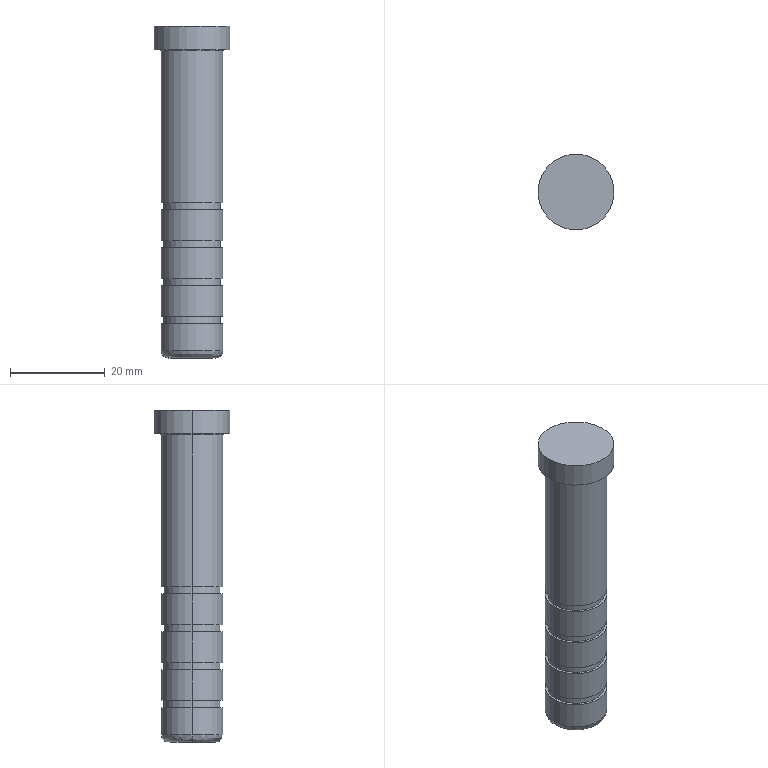Part | STEP file | SGOH13-70 | 1 solid | 35 faces | box 16 x 16 x 70 mm | volume 9500 mm3 | cylinder 20 | plane 11 | spline 4 | commonest cylinder face diameters 13 x10 12 x8 16 x2
STEP:
#1=CARTESIAN_POINT('',(6.75,0.,0.));
#2=VERTEX_POINT('',#1);
#3=CARTESIAN_POINT('',(-6.75,0.,0.));
#4=VERTEX_POINT('',#3);
#5=CARTESIAN_POINT('',(6.75,0.,0.));
#6=CARTESIAN_POINT('',(6.75,0.2065,0.));
#7=CARTESIAN_POINT('',(6.736,0.5149,0.));
#8=CARTESIAN_POINT('',(6.695,0.8724,0.));
#9=CARTESIAN_POINT('',(6.668,1.051,0.));
#10=CARTESIAN_POINT('',(6.655,1.127,0.));
#11=CARTESIAN_POINT('',(6.647,1.178,0.));
#12=CARTESIAN_POINT('',(6.642,1.201,0.));
#13=CARTESIAN_POINT('',(6.598,1.443,0.));
#14=CARTESIAN_POINT('',(6.523,1.762,0.));
#15=CARTESIAN_POINT('',(6.408,2.126,0.));
#16=CARTESIAN_POINT('',(6.354,2.28,0.));
#17=CARTESIAN_POINT('',(6.316,2.383,0.));
#18=CARTESIAN_POINT('',(6.297,2.432,0.));
#19=CARTESIAN_POINT('',(6.192,2.697,0.));
#20=CARTESIAN_POINT('',(6.051,3.007,0.));
#21=CARTESIAN_POINT('',(5.859,3.355,0.));
#22=CARTESIAN_POINT('',(5.771,3.501,0.));
#23=CARTESIAN_POINT('',(5.712,3.598,0.));
#24=CARTESIAN_POINT('',(5.682,3.645,0.));
#25=CARTESIAN_POINT('',(5.395,4.083,0.));
#26=CARTESIAN_POINT('',(5.102,4.444,0.));
#27=CARTESIAN_POINT('',(4.608,4.938,0.));
#28=CARTESIAN_POINT('',(4.35,5.171,0.));
#29=CARTESIAN_POINT('',(4.029,5.418,0.));
#30=CARTESIAN_POINT('',(3.886,5.519,0.));
#31=CARTESIAN_POINT('',(3.791,5.585,0.));
#32=CARTESIAN_POINT('',(3.741,5.619,0.));
#33=CARTESIAN_POINT('',(3.503,5.774,0.));
#34=CARTESIAN_POINT('',(3.209,5.946,0.));
#35=CARTESIAN_POINT('',(2.851,6.12,0.));
#36=CARTESIAN_POINT('',(2.669,6.2,0.));
#37=CARTESIAN_POINT('',(2.59,6.233,0.));
#38=CARTESIAN_POINT('',(2.538,6.255,0.));
#39=CARTESIAN_POINT('',(2.51,6.266,0.));
#40=CARTESIAN_POINT('',(2.281,6.357,0.));
#41=CARTESIAN_POINT('',(1.972,6.462,0.));
#42=CARTESIAN_POINT('',(1.603,6.559,0.));
#43=CARTESIAN_POINT('',(1.416,6.6,0.));
#44=CARTESIAN_POINT('',(1.336,6.617,0.));
#45=CARTESIAN_POINT('',(1.282,6.627,0.));
#46=CARTESIAN_POINT('',(1.254,6.633,0.));
#47=CARTESIAN_POINT('',(0.8226,6.712,0.));
#48=CARTESIAN_POINT('',(0.4125,6.75,0.));
#49=CARTESIAN_POINT('',(-0.2063,6.75,0.));
#50=CARTESIAN_POINT('',(-0.5145,6.736,0.));
#51=CARTESIAN_POINT('',(-0.872,6.695,0.));
#52=CARTESIAN_POINT('',(-1.05,6.668,0.));
#53=CARTESIAN_POINT('',(-1.127,6.655,0.));
#54=CARTESIAN_POINT('',(-1.177,6.647,0.));
#55=CARTESIAN_POINT('',(-1.201,6.642,0.));
#56=CARTESIAN_POINT('',(-1.443,6.598,0.));
#57=CARTESIAN_POINT('',(-1.762,6.523,0.));
#58=CARTESIAN_POINT('',(-2.126,6.408,0.));
#59=CARTESIAN_POINT('',(-2.28,6.354,0.));
#60=CARTESIAN_POINT('',(-2.383,6.316,0.));
#61=CARTESIAN_POINT('',(-2.432,6.297,0.));
#62=CARTESIAN_POINT('',(-2.697,6.192,0.));
#63=CARTESIAN_POINT('',(-3.007,6.051,0.));
#64=CARTESIAN_POINT('',(-3.355,5.859,0.));
#65=CARTESIAN_POINT('',(-3.501,5.771,0.));
#66=CARTESIAN_POINT('',(-3.598,5.712,0.));
#67=CARTESIAN_POINT('',(-3.645,5.682,0.));
#68=CARTESIAN_POINT('',(-4.083,5.395,0.));
#69=CARTESIAN_POINT('',(-4.444,5.102,0.));
#70=CARTESIAN_POINT('',(-4.938,4.608,0.));
#71=CARTESIAN_POINT('',(-5.171,4.35,0.));
#72=CARTESIAN_POINT('',(-5.418,4.029,0.));
#73=CARTESIAN_POINT('',(-5.519,3.886,0.));
#74=CARTESIAN_POINT('',(-5.585,3.791,0.));
#75=CARTESIAN_POINT('',(-5.619,3.741,0.));
#76=CARTESIAN_POINT('',(-5.774,3.503,0.));
#77=CARTESIAN_POINT('',(-5.946,3.209,0.));
#78=CARTESIAN_POINT('',(-6.12,2.851,0.));
#79=CARTESIAN_POINT('',(-6.2,2.669,0.));
#80=CARTESIAN_POINT('',(-6.233,2.59,0.));
#81=CARTESIAN_POINT('',(-6.255,2.538,0.));
#82=CARTESIAN_POINT('',(-6.266,2.51,0.));
#83=CARTESIAN_POINT('',(-6.357,2.281,0.));
#84=CARTESIAN_POINT('',(-6.462,1.972,0.));
#85=CARTESIAN_POINT('',(-6.559,1.603,0.));
#86=CARTESIAN_POINT('',(-6.6,1.416,0.));
#87=CARTESIAN_POINT('',(-6.617,1.336,0.));
#88=CARTESIAN_POINT('',(-6.627,1.282,0.));
#89=CARTESIAN_POINT('',(-6.633,1.254,0.));
#90=CARTESIAN_POINT('',(-6.712,0.8228,0.));
#91=CARTESIAN_POINT('',(-6.75,0.4134,0.));
#92=CARTESIAN_POINT('',(-6.75,0.,0.));
#93=B_SPLINE_CURVE_WITH_KNOTS('',3,(#5,#6,#7,#8,#9,#10,#11,#12,#13,#14,#15,#16,#17,#18,#19,#20,#21,#22,#23,#24,#25,#26,#27,#28,#29,#30,#31,#32,#33,#34,#35,#36,#37,#38,#39,#40,#41,#42,#43,#44,#45,#46,#47,#48,#49,#50,#51,#52,#53,#54,#55,#56,#57,#58,#59,#60,#61,#62,#63,#64,#65,#66,#67,#68,#69,#70,#71,#72,#73,#74,#75,#76,#77,#78,#79,#80,#81,#82,#83,#84,#85,#86,#87,#88,#89,#90,#91,#92),.UNSPECIFIED.,.F.,.F.,(4,1,1,1,2,2,1,1,2,2,1,1,2,2,2,1,1,2,2,1,1,1,2,2,1,1,1,2,2,2,1,1,1,2,2,1,1,2,2,1,1,2,2,2,1,1,2,2,1,1,1,2,2,1,1,1,2,2,4),(0.,0.03125,0.04687,0.05469,0.05859,0.0625,0.09375,0.1094,0.1172,0.125,0.1562,0.1719,0.1797,0.1875,0.25,0.2812,0.2969,0.3047,0.3125,0.3437,0.3594,0.3672,0.3711,0.375,0.4062,0.4219,0.4297,0.4336,0.4375,0.5,0.5312,0.5469,0.5547,0.5586,0.5625,0.5937,0.6094,0.6172,0.625,0.6563,0.6719,0.6797,0.6875,0.75,0.7813,0.7969,0.8047,0.8125,0.8438,0.8594,0.8672,0.8711,0.875,0.9063,0.9219,0.9297,0.9336,0.9375,1.),.UNSPECIFIED.);
#94=EDGE_CURVE('',#2,#4,#93,.T.);
#95=ORIENTED_EDGE('',*,*,#94,.F.);
#96=CARTESIAN_POINT('',(6.5,0.,-0.25));
#97=VERTEX_POINT('',#96);
#98=CARTESIAN_POINT('',(6.75,0.,-0.25));
#99=DIRECTION('',(0.,-1.,0.));
#100=DIRECTION('',(1.,0.,0.));
#101=AXIS2_PLACEMENT_3D('',#98,#99,#100);
#102=CIRCLE('',#101,0.25);
#103=EDGE_CURVE('',#2,#97,#102,.T.);
#104=ORIENTED_EDGE('',*,*,#103,.T.);
#105=CARTESIAN_POINT('',(-6.5,0.,-0.25));
#106=VERTEX_POINT('',#105);
#107=CARTESIAN_POINT('',(0.,0.,-0.25));
#108=DIRECTION('',(0.,0.,-1.));
#109=DIRECTION('',(-1.,0.,0.));
#110=AXIS2_PLACEMENT_3D('',#107,#108,#109);
#111=CIRCLE('',#110,6.5);
#112=EDGE_CURVE('',#106,#97,#111,.T.);
#113=ORIENTED_EDGE('',*,*,#112,.F.);
#114=CARTESIAN_POINT('',(-6.75,0.,-0.25));
#115=DIRECTION('',(0.,1.,0.));
#116=DIRECTION('',(-1.,0.,0.));
#117=AXIS2_PLACEMENT_3D('',#114,#115,#116);
#118=CIRCLE('',#117,0.25);
#119=EDGE_CURVE('',#4,#106,#118,.T.);
#120=ORIENTED_EDGE('',*,*,#119,.F.);
#121=EDGE_LOOP('',(#95,#104,#113,#120));
#122=FACE_OUTER_BOUND('',#121,.T.);
#123=CARTESIAN_POINT('',(-6.75,0.,0.));
#124=CARTESIAN_POINT('',(-6.75,13.5,0.));
#125=CARTESIAN_POINT('',(6.75,13.5,0.));
#126=CARTESIAN_POINT('',(6.75,0.,0.));
#127=CARTESIAN_POINT('',(-6.604,0.,0.));
#128=CARTESIAN_POINT('',(-6.604,13.207,0.));
#129=CARTESIAN_POINT('',(6.604,13.207,0.));
#130=CARTESIAN_POINT('',(6.604,0.,0.));
#131=CARTESIAN_POINT('',(-6.5,0.,-0.1036));
#132=CARTESIAN_POINT('',(-6.5,13.,-0.1036));
#133=CARTESIAN_POINT('',(6.5,13.,-0.1036));
#134=CARTESIAN_POINT('',(6.5,0.,-0.1036));
#135=CARTESIAN_POINT('',(-6.5,0.,-0.25));
#136=CARTESIAN_POINT('',(-6.5,13.,-0.25));
#137=CARTESIAN_POINT('',(6.5,13.,-0.25));
#138=CARTESIAN_POINT('',(6.5,0.,-0.25));
#139=(BOUNDED_SURFACE()B_SPLINE_SURFACE(3,3,((#123,#124,#125,#126),(#127,#128,#129,#130),(#131,#132,#133,#134),(#135,#136,#137,#138)),.UNSPECIFIED.,.F.,.F.,.F.)B_SPLINE_SURFACE_WITH_KNOTS((4,4),(4,4),(0.,1.),(0.,1.),.UNSPECIFIED.)GEOMETRIC_REPRESENTATION_ITEM()RATIONAL_B_SPLINE_SURFACE(((1.,0.3333,0.3333,1.),(0.8047,0.2682,0.2682,0.8047),(0.8047,0.2682,0.2682,0.8047),(1.,0.3333,0.3333,1.)))REPRESENTATION_ITEM('')SURFACE());
#140=ADVANCED_FACE('',(#122),#139,.F.);
#141=CARTESIAN_POINT('',(-5.,0.,-65.));
#142=VERTEX_POINT('',#141);
#143=CARTESIAN_POINT('',(5.,0.,-65.));
#144=VERTEX_POINT('',#143);
#145=CARTESIAN_POINT('',(-5.,0.,-65.));
#146=CARTESIAN_POINT('',(-5.,-10.,-65.));
#147=CARTESIAN_POINT('',(5.,-10.,-65.));
#148=CARTESIAN_POINT('',(5.,0.,-65.));
#149=(BOUNDED_CURVE()B_SPLINE_CURVE(3,(#145,#146,#147,#148),.UNSPECIFIED.,.F.,.F.)B_SPLINE_CURVE_WITH_KNOTS((4,4),(0.,1.),.UNSPECIFIED.)CURVE()GEOMETRIC_REPRESENTATION_ITEM()RATIONAL_B_SPLINE_CURVE((1.,0.3333,0.3333,1.))REPRESENTATION_ITEM(''));
#150=EDGE_CURVE('',#142,#144,#149,.T.);
#151=ORIENTED_EDGE('',*,*,#150,.T.);
#152=CARTESIAN_POINT('',(6.5,0.,-63.5));
#153=VERTEX_POINT('',#152);
#154=CARTESIAN_POINT('',(5.,0.,-63.5));
#155=DIRECTION('',(0.,-1.,0.));
#156=DIRECTION('',(1.,0.,0.));
#157=AXIS2_PLACEMENT_3D('',#154,#155,#156);
#158=CIRCLE('',#157,1.5);
#159=EDGE_CURVE('',#144,#153,#158,.T.);
#160=ORIENTED_EDGE('',*,*,#159,.T.);
#161=CARTESIAN_POINT('',(-6.5,0.,-63.5));
#162=VERTEX_POINT('',#161);
#163=CARTESIAN_POINT('',(0.,0.,-63.5));
#164=DIRECTION('',(0.,0.,1.));
#165=DIRECTION('',(-1.,0.,0.));
#166=AXIS2_PLACEMENT_3D('',#163,#164,#165);
#167=CIRCLE('',#166,6.5);
#168=EDGE_CURVE('',#162,#153,#167,.T.);
#169=ORIENTED_EDGE('',*,*,#168,.F.);
#170=CARTESIAN_POINT('',(-5.,0.,-63.5));
#171=DIRECTION('',(0.,1.,0.));
#172=DIRECTION('',(-1.,0.,0.));
#173=AXIS2_PLACEMENT_3D('',#170,#171,#172);
#174=CIRCLE('',#173,1.5);
#175=EDGE_CURVE('',#142,#162,#174,.T.);
#176=ORIENTED_EDGE('',*,*,#175,.F.);
#177=EDGE_LOOP('',(#151,#160,#169,#176));
#178=FACE_OUTER_BOUND('',#177,.T.);
#179=CARTESIAN_POINT('',(5.,0.,-65.));
#180=CARTESIAN_POINT('',(5.,-10.,-65.));
#181=CARTESIAN_POINT('',(-5.,-10.,-65.));
#182=CARTESIAN_POINT('',(-5.,0.,-65.));
#183=CARTESIAN_POINT('',(5.879,0.,-65.));
#184=CARTESIAN_POINT('',(5.879,-11.757,-65.));
#185=CARTESIAN_POINT('',(-5.879,-11.757,-65.));
#186=CARTESIAN_POINT('',(-5.879,0.,-65.));
#187=CARTESIAN_POINT('',(6.5,0.,-64.379));
#188=CARTESIAN_POINT('',(6.5,-13.,-64.379));
#189=CARTESIAN_POINT('',(-6.5,-13.,-64.379));
#190=CARTESIAN_POINT('',(-6.5,0.,-64.379));
#191=CARTESIAN_POINT('',(6.5,0.,-63.5));
#192=CARTESIAN_POINT('',(6.5,-13.,-63.5));
#193=CARTESIAN_POINT('',(-6.5,-13.,-63.5));
#194=CARTESIAN_POINT('',(-6.5,0.,-63.5));
#195=(BOUNDED_SURFACE()B_SPLINE_SURFACE(3,3,((#179,#180,#181,#182),(#183,#184,#185,#186),(#187,#188,#189,#190),(#191,#192,#193,#194)),.UNSPECIFIED.,.F.,.F.,.F.)B_SPLINE_SURFACE_WITH_KNOTS((4,4),(4,4),(0.,1.),(0.,1.),.UNSPECIFIED.)GEOMETRIC_REPRESENTATION_ITEM()RATIONAL_B_SPLINE_SURFACE(((1.,0.3333,0.3333,1.),(0.8047,0.2682,0.2682,0.8047),(0.8047,0.2682,0.2682,0.8047),(1.,0.3333,0.3333,1.)))REPRESENTATION_ITEM('')SURFACE());
#196=ADVANCED_FACE('',(#178),#195,.T.);
#197=ORIENTED_EDGE('',*,*,#112,.T.);
#198=CARTESIAN_POINT('',(6.5,0.,-32.25));
#199=VERTEX_POINT('',#198);
#200=CARTESIAN_POINT('',(6.5,0.,-16.));
#201=DIRECTION('',(0.,0.,-1.));
#202=VECTOR('',#201,1000.);
#203=LINE('',#200,#202);
#204=EDGE_CURVE('',#97,#199,#203,.T.);
#205=ORIENTED_EDGE('',*,*,#204,.T.);
#206=CARTESIAN_POINT('',(-6.5,0.,-32.25));
#207=VERTEX_POINT('',#206);
#208=CARTESIAN_POINT('',(0.,0.,-32.25));
#209=DIRECTION('',(0.,0.,1.));
#210=DIRECTION('',(-1.,0.,0.));
#211=AXIS2_PLACEMENT_3D('',#208,#209,#210);
#212=CIRCLE('',#211,6.5);
#213=EDGE_CURVE('',#199,#207,#212,.T.);
#214=ORIENTED_EDGE('',*,*,#213,.T.);
#215=CARTESIAN_POINT('',(-6.5,0.,-16.));
#216=DIRECTION('',(0.,0.,-1.));
#217=VECTOR('',#216,1000.);
#218=LINE('',#215,#217);
#219=EDGE_CURVE('',#106,#207,#218,.T.);
#220=ORIENTED_EDGE('',*,*,#219,.F.);
#221=EDGE_LOOP('',(#197,#205,#214,#220));
#222=FACE_OUTER_BOUND('',#221,.T.);
#223=CARTESIAN_POINT('',(0.,0.,-16.));
#224=DIRECTION('',(0.,0.,-1.));
#225=DIRECTION('',(-1.,0.,0.));
#226=AXIS2_PLACEMENT_3D('',#223,#224,#225);
#227=CYLINDRICAL_SURFACE('',#226,6.5);
#228=ADVANCED_FACE('',(#222),#227,.T.);
#229=CARTESIAN_POINT('',(-6.,0.,-32.25));
#230=VERTEX_POINT('',#229);
#231=CARTESIAN_POINT('',(6.,0.,-32.25));
#232=VERTEX_POINT('',#231);
#233=CARTESIAN_POINT('',(0.,0.,-32.25));
#234=DIRECTION('',(0.,0.,-1.));
#235=DIRECTION('',(-1.,0.,0.));
#236=AXIS2_PLACEMENT_3D('',#233,#234,#235);
#237=CIRCLE('',#236,6.);
#238=EDGE_CURVE('',#230,#232,#237,.T.);
#239=ORIENTED_EDGE('',*,*,#238,.T.);
#240=CARTESIAN_POINT('',(6.,0.,-33.75));
#241=VERTEX_POINT('',#240);
#242=CARTESIAN_POINT('',(6.,0.,-32.25));
#243=DIRECTION('',(0.,0.,-1.));
#244=VECTOR('',#243,1000.);
#245=LINE('',#242,#244);
#246=EDGE_CURVE('',#232,#241,#245,.T.);
#247=ORIENTED_EDGE('',*,*,#246,.T.);
#248=CARTESIAN_POINT('',(-6.,0.,-33.75));
#249=VERTEX_POINT('',#248);
#250=CARTESIAN_POINT('',(0.,0.,-33.75));
#251=DIRECTION('',(0.,0.,1.));
#252=DIRECTION('',(-1.,0.,0.));
#253=AXIS2_PLACEMENT_3D('',#250,#251,#252);
#254=CIRCLE('',#253,6.);
#255=EDGE_CURVE('',#241,#249,#254,.T.);
#256=ORIENTED_EDGE('',*,*,#255,.T.);
#257=CARTESIAN_POINT('',(-6.,0.,-32.25));
#258=DIRECTION('',(0.,0.,-1.));
#259=VECTOR('',#258,1000.);
#260=LINE('',#257,#259);
#261=EDGE_CURVE('',#230,#249,#260,.T.);
#262=ORIENTED_EDGE('',*,*,#261,.F.);
#263=EDGE_LOOP('',(#239,#247,#256,#262));
#264=FACE_OUTER_BOUND('',#263,.T.);
#265=CARTESIAN_POINT('',(0.,0.,-32.25));
#266=DIRECTION('',(0.,0.,-1.));
#267=DIRECTION('',(-1.,0.,0.));
#268=AXIS2_PLACEMENT_3D('',#265,#266,#267);
#269=CYLINDRICAL_SURFACE('',#268,6.);
#270=ADVANCED_FACE('',(#264),#269,.T.);
#271=CARTESIAN_POINT('',(-8.,0.,5.));
#272=VERTEX_POINT('',#271);
#273=CARTESIAN_POINT('',(8.,0.,5.));
#274=VERTEX_POINT('',#273);
#275=CARTESIAN_POINT('',(0.,0.,5.));
#276=DIRECTION('',(0.,0.,-1.));
#277=DIRECTION('',(-1.,0.,0.));
#278=AXIS2_PLACEMENT_3D('',#275,#276,#277);
#279=CIRCLE('',#278,8.);
#280=EDGE_CURVE('',#272,#274,#279,.T.);
#281=ORIENTED_EDGE('',*,*,#280,.T.);
#282=CARTESIAN_POINT('',(8.,0.,0.));
#283=VERTEX_POINT('',#282);
#284=CARTESIAN_POINT('',(8.,0.,5.));
#285=DIRECTION('',(0.,0.,-1.));
#286=VECTOR('',#285,1000.);
#287=LINE('',#284,#286);
#288=EDGE_CURVE('',#274,#283,#287,.T.);
#289=ORIENTED_EDGE('',*,*,#288,.T.);
#290=CARTESIAN_POINT('',(-8.,0.,0.));
#291=VERTEX_POINT('',#290);
#292=CARTESIAN_POINT('',(0.,0.,0.));
#293=DIRECTION('',(0.,0.,-1.));
#294=DIRECTION('',(-1.,0.,0.));
#295=AXIS2_PLACEMENT_3D('',#292,#293,#294);
#296=CIRCLE('',#295,8.);
#297=EDGE_CURVE('',#291,#283,#296,.T.);
#298=ORIENTED_EDGE('',*,*,#297,.F.);
#299=CARTESIAN_POINT('',(-8.,0.,5.));
#300=DIRECTION('',(0.,0.,-1.));
#301=VECTOR('',#300,1000.);
#302=LINE('',#299,#301);
#303=EDGE_CURVE('',#272,#291,#302,.T.);
#304=ORIENTED_EDGE('',*,*,#303,.F.);
#305=EDGE_LOOP('',(#281,#289,#298,#304));
#306=FACE_OUTER_BOUND('',#305,.T.);
#307=CARTESIAN_POINT('',(0.,0.,5.));
#308=DIRECTION('',(0.,0.,-1.));
#309=DIRECTION('',(-1.,0.,0.));
#310=AXIS2_PLACEMENT_3D('',#307,#308,#309);
#311=CYLINDRICAL_SURFACE('',#310,8.);
#312=ADVANCED_FACE('',(#306),#311,.T.);
#313=CARTESIAN_POINT('',(-6.5,0.,-33.75));
#314=VERTEX_POINT('',#313);
#315=CARTESIAN_POINT('',(6.5,0.,-33.75));
#316=VERTEX_POINT('',#315);
#317=CARTESIAN_POINT('',(0.,0.,-33.75));
#318=DIRECTION('',(0.,0.,-1.));
#319=DIRECTION('',(-1.,0.,0.));
#320=AXIS2_PLACEMENT_3D('',#317,#318,#319);
#321=CIRCLE('',#320,6.5);
#322=EDGE_CURVE('',#314,#316,#321,.T.);
#323=ORIENTED_EDGE('',*,*,#322,.T.);
#324=CARTESIAN_POINT('',(6.5,0.,-40.25));
#325=VERTEX_POINT('',#324);
#326=CARTESIAN_POINT('',(6.5,0.,-16.));
#327=DIRECTION('',(0.,0.,-1.));
#328=VECTOR('',#327,1000.);
#329=LINE('',#326,#328);
#330=EDGE_CURVE('',#316,#325,#329,.T.);
#331=ORIENTED_EDGE('',*,*,#330,.T.);
#332=CARTESIAN_POINT('',(-6.5,0.,-40.25));
#333=VERTEX_POINT('',#332);
#334=CARTESIAN_POINT('',(0.,0.,-40.25));
#335=DIRECTION('',(0.,0.,1.));
#336=DIRECTION('',(-1.,0.,0.));
#337=AXIS2_PLACEMENT_3D('',#334,#335,#336);
#338=CIRCLE('',#337,6.5);
#339=EDGE_CURVE('',#325,#333,#338,.T.);
#340=ORIENTED_EDGE('',*,*,#339,.T.);
#341=CARTESIAN_POINT('',(-6.5,0.,-16.));
#342=DIRECTION('',(0.,0.,-1.));
#343=VECTOR('',#342,1000.);
#344=LINE('',#341,#343);
#345=EDGE_CURVE('',#314,#333,#344,.T.);
#346=ORIENTED_EDGE('',*,*,#345,.F.);
#347=EDGE_LOOP('',(#323,#331,#340,#346));
#348=FACE_OUTER_BOUND('',#347,.T.);
#349=CARTESIAN_POINT('',(0.,0.,-16.));
#350=DIRECTION('',(0.,0.,-1.));
#351=DIRECTION('',(-1.,0.,0.));
#352=AXIS2_PLACEMENT_3D('',#349,#350,#351);
#353=CYLINDRICAL_SURFACE('',#352,6.5);
#354=ADVANCED_FACE('',(#348),#353,.T.);
#355=CARTESIAN_POINT('',(-6.,0.,-40.25));
#356=VERTEX_POINT('',#355);
#357=CARTESIAN_POINT('',(6.,0.,-40.25));
#358=VERTEX_POINT('',#357);
#359=CARTESIAN_POINT('',(0.,0.,-40.25));
#360=DIRECTION('',(0.,0.,-1.));
#361=DIRECTION('',(-1.,0.,0.));
#362=AXIS2_PLACEMENT_3D('',#359,#360,#361);
#363=CIRCLE('',#362,6.);
#364=EDGE_CURVE('',#356,#358,#363,.T.);
#365=ORIENTED_EDGE('',*,*,#364,.T.);
#366=CARTESIAN_POINT('',(6.,0.,-41.75));
#367=VERTEX_POINT('',#366);
#368=CARTESIAN_POINT('',(6.,0.,-40.25));
#369=DIRECTION('',(0.,0.,-1.));
#370=VECTOR('',#369,1000.);
#371=LINE('',#368,#370);
#372=EDGE_CURVE('',#358,#367,#371,.T.);
#373=ORIENTED_EDGE('',*,*,#372,.T.);
#374=CARTESIAN_POINT('',(-6.,0.,-41.75));
#375=VERTEX_POINT('',#374);
#376=CARTESIAN_POINT('',(0.,0.,-41.75));
#377=DIRECTION('',(0.,0.,1.));
#378=DIRECTION('',(-1.,0.,0.));
#379=AXIS2_PLACEMENT_3D('',#376,#377,#378);
#380=CIRCLE('',#379,6.);
#381=EDGE_CURVE('',#367,#375,#380,.T.);
#382=ORIENTED_EDGE('',*,*,#381,.T.);
#383=CARTESIAN_POINT('',(-6.,0.,-40.25));
#384=DIRECTION('',(0.,0.,-1.));
#385=VECTOR('',#384,1000.);
#386=LINE('',#383,#385);
#387=EDGE_CURVE('',#356,#375,#386,.T.);
#388=ORIENTED_EDGE('',*,*,#387,.F.);
#389=EDGE_LOOP('',(#365,#373,#382,#388));
#390=FACE_OUTER_BOUND('',#389,.T.);
#391=CARTESIAN_POINT('',(0.,0.,-40.25));
#392=DIRECTION('',(0.,0.,-1.));
#393=DIRECTION('',(-1.,0.,0.));
#394=AXIS2_PLACEMENT_3D('',#391,#392,#393);
#395=CYLINDRICAL_SURFACE('',#394,6.);
#396=ADVANCED_FACE('',(#390),#395,.T.);
#397=CARTESIAN_POINT('',(-6.5,0.,-41.75));
#398=VERTEX_POINT('',#397);
#399=CARTESIAN_POINT('',(6.5,0.,-41.75));
#400=VERTEX_POINT('',#399);
#401=CARTESIAN_POINT('',(0.,0.,-41.75));
#402=DIRECTION('',(0.,0.,-1.));
#403=DIRECTION('',(-1.,0.,0.));
#404=AXIS2_PLACEMENT_3D('',#401,#402,#403);
#405=CIRCLE('',#404,6.5);
#406=EDGE_CURVE('',#398,#400,#405,.T.);
#407=ORIENTED_EDGE('',*,*,#406,.T.);
#408=CARTESIAN_POINT('',(6.5,0.,-48.25));
#409=VERTEX_POINT('',#408);
#410=CARTESIAN_POINT('',(6.5,0.,-16.));
#411=DIRECTION('',(0.,0.,-1.));
#412=VECTOR('',#411,1000.);
#413=LINE('',#410,#412);
#414=EDGE_CURVE('',#400,#409,#413,.T.);
#415=ORIENTED_EDGE('',*,*,#414,.T.);
#416=CARTESIAN_POINT('',(-6.5,0.,-48.25));
#417=VERTEX_POINT('',#416);
#418=CARTESIAN_POINT('',(0.,0.,-48.25));
#419=DIRECTION('',(0.,0.,1.));
#420=DIRECTION('',(-1.,0.,0.));
#421=AXIS2_PLACEMENT_3D('',#418,#419,#420);
#422=CIRCLE('',#421,6.5);
#423=EDGE_CURVE('',#409,#417,#422,.T.);
#424=ORIENTED_EDGE('',*,*,#423,.T.);
#425=CARTESIAN_POINT('',(-6.5,0.,-16.));
#426=DIRECTION('',(0.,0.,-1.));
#427=VECTOR('',#426,1000.);
#428=LINE('',#425,#427);
#429=EDGE_CURVE('',#398,#417,#428,.T.);
#430=ORIENTED_EDGE('',*,*,#429,.F.);
#431=EDGE_LOOP('',(#407,#415,#424,#430));
#432=FACE_OUTER_BOUND('',#431,.T.);
#433=CARTESIAN_POINT('',(0.,0.,-16.));
#434=DIRECTION('',(0.,0.,-1.));
#435=DIRECTION('',(-1.,0.,0.));
#436=AXIS2_PLACEMENT_3D('',#433,#434,#435);
#437=CYLINDRICAL_SURFACE('',#436,6.5);
#438=ADVANCED_FACE('',(#432),#437,.T.);
#439=CARTESIAN_POINT('',(6.,0.,-48.25));
#440=VERTEX_POINT('',#439);
#441=CARTESIAN_POINT('',(-6.,0.,-48.25));
#442=VERTEX_POINT('',#441);
#443=CARTESIAN_POINT('',(0.,0.,-48.25));
#444=DIRECTION('',(0.,0.,1.));
#445=DIRECTION('',(-1.,0.,0.));
#446=AXIS2_PLACEMENT_3D('',#443,#444,#445);
#447=CIRCLE('',#446,6.);
#448=EDGE_CURVE('',#440,#442,#447,.T.);
#449=ORIENTED_EDGE('',*,*,#448,.F.);
#450=CARTESIAN_POINT('',(6.,0.,-49.75));
#451=VERTEX_POINT('',#450);
#452=CARTESIAN_POINT('',(6.,0.,-48.25));
#453=DIRECTION('',(0.,0.,-1.));
#454=VECTOR('',#453,1000.);
#455=LINE('',#452,#454);
#456=EDGE_CURVE('',#440,#451,#455,.T.);
#457=ORIENTED_EDGE('',*,*,#456,.T.);
#458=CARTESIAN_POINT('',(-6.,0.,-49.75));
#459=VERTEX_POINT('',#458);
#460=CARTESIAN_POINT('',(0.,0.,-49.75));
#461=DIRECTION('',(0.,0.,1.));
#462=DIRECTION('',(-1.,0.,0.));
#463=AXIS2_PLACEMENT_3D('',#460,#461,#462);
#464=CIRCLE('',#463,6.);
#465=EDGE_CURVE('',#451,#459,#464,.T.);
#466=ORIENTED_EDGE('',*,*,#465,.T.);
#467=CARTESIAN_POINT('',(-6.,0.,-48.25));
#468=DIRECTION('',(0.,0.,-1.));
#469=VECTOR('',#468,1000.);
#470=LINE('',#467,#469);
#471=EDGE_CURVE('',#442,#459,#470,.T.);
#472=ORIENTED_EDGE('',*,*,#471,.F.);
#473=EDGE_LOOP('',(#449,#457,#466,#472));
#474=FACE_OUTER_BOUND('',#473,.T.);
#475=CARTESIAN_POINT('',(0.,0.,-48.25));
#476=DIRECTION('',(0.,0.,-1.));
#477=DIRECTION('',(-1.,0.,0.));
#478=AXIS2_PLACEMENT_3D('',#475,#476,#477);
#479=CYLINDRICAL_SURFACE('',#478,6.);
#480=ADVANCED_FACE('',(#474),#479,.T.);
#481=CARTESIAN_POINT('',(6.5,0.,-49.75));
#482=VERTEX_POINT('',#481);
#483=CARTESIAN_POINT('',(-6.5,0.,-49.75));
#484=VERTEX_POINT('',#483);
#485=CARTESIAN_POINT('',(0.,0.,-49.75));
#486=DIRECTION('',(0.,0.,1.));
#487=DIRECTION('',(-1.,0.,0.));
#488=AXIS2_PLACEMENT_3D('',#485,#486,#487);
#489=CIRCLE('',#488,6.5);
#490=EDGE_CURVE('',#482,#484,#489,.T.);
#491=ORIENTED_EDGE('',*,*,#490,.F.);
#492=CARTESIAN_POINT('',(6.5,0.,-56.25));
#493=VERTEX_POINT('',#492);
#494=CARTESIAN_POINT('',(6.5,0.,-49.75));
#495=DIRECTION('',(0.,0.,-1.));
#496=VECTOR('',#495,1000.);
#497=LINE('',#494,#496);
#498=EDGE_CURVE('',#482,#493,#497,.T.);
#499=ORIENTED_EDGE('',*,*,#498,.T.);
#500=CARTESIAN_POINT('',(-6.5,0.,-56.25));
#501=VERTEX_POINT('',#500);
#502=CARTESIAN_POINT('',(0.,0.,-56.25));
#503=DIRECTION('',(0.,0.,1.));
#504=DIRECTION('',(-1.,0.,0.));
#505=AXIS2_PLACEMENT_3D('',#502,#503,#504);
#506=CIRCLE('',#505,6.5);
#507=EDGE_CURVE('',#493,#501,#506,.T.);
#508=ORIENTED_EDGE('',*,*,#507,.T.);
#509=CARTESIAN_POINT('',(-6.5,0.,-49.75));
#510=DIRECTION('',(0.,0.,-1.));
#511=VECTOR('',#510,1000.);
#512=LINE('',#509,#511);
#513=EDGE_CURVE('',#484,#501,#512,.T.);
#514=ORIENTED_EDGE('',*,*,#513,.F.);
#515=EDGE_LOOP('',(#491,#499,#508,#514));
#516=FACE_OUTER_BOUND('',#515,.T.);
#517=CARTESIAN_POINT('',(0.,0.,-49.75));
#518=DIRECTION('',(0.,0.,-1.));
#519=DIRECTION('',(-1.,0.,0.));
#520=AXIS2_PLACEMENT_3D('',#517,#518,#519);
#521=CYLINDRICAL_SURFACE('',#520,6.5);
#522=ADVANCED_FACE('',(#516),#521,.T.);
#523=CARTESIAN_POINT('',(6.,0.,-56.25));
#524=VERTEX_POINT('',#523);
#525=CARTESIAN_POINT('',(-6.,0.,-56.25));
#526=VERTEX_POINT('',#525);
#527=CARTESIAN_POINT('',(0.,0.,-56.25));
#528=DIRECTION('',(0.,0.,1.));
#529=DIRECTION('',(-1.,0.,0.));
#530=AXIS2_PLACEMENT_3D('',#527,#528,#529);
#531=CIRCLE('',#530,6.);
#532=EDGE_CURVE('',#524,#526,#531,.T.);
#533=ORIENTED_EDGE('',*,*,#532,.F.);
#534=CARTESIAN_POINT('',(6.,0.,-57.75));
#535=VERTEX_POINT('',#534);
#536=CARTESIAN_POINT('',(6.,0.,-56.25));
#537=DIRECTION('',(0.,0.,-1.));
#538=VECTOR('',#537,1000.);
#539=LINE('',#536,#538);
#540=EDGE_CURVE('',#524,#535,#539,.T.);
#541=ORIENTED_EDGE('',*,*,#540,.T.);
#542=CARTESIAN_POINT('',(-6.,0.,-57.75));
#543=VERTEX_POINT('',#542);
#544=CARTESIAN_POINT('',(0.,0.,-57.75));
#545=DIRECTION('',(0.,0.,1.));
#546=DIRECTION('',(-1.,0.,0.));
#547=AXIS2_PLACEMENT_3D('',#544,#545,#546);
#548=CIRCLE('',#547,6.);
#549=EDGE_CURVE('',#535,#543,#548,.T.);
#550=ORIENTED_EDGE('',*,*,#549,.T.);
#551=CARTESIAN_POINT('',(-6.,0.,-56.25));
#552=DIRECTION('',(0.,0.,-1.));
#553=VECTOR('',#552,1000.);
#554=LINE('',#551,#553);
#555=EDGE_CURVE('',#526,#543,#554,.T.);
#556=ORIENTED_EDGE('',*,*,#555,.F.);
#557=EDGE_LOOP('',(#533,#541,#550,#556));
#558=FACE_OUTER_BOUND('',#557,.T.);
#559=CARTESIAN_POINT('',(0.,0.,-56.25));
#560=DIRECTION('',(0.,0.,-1.));
#561=DIRECTION('',(-1.,0.,0.));
#562=AXIS2_PLACEMENT_3D('',#559,#560,#561);
#563=CYLINDRICAL_SURFACE('',#562,6.);
#564=ADVANCED_FACE('',(#558),#563,.T.);
#565=CARTESIAN_POINT('',(6.5,0.,-57.75));
#566=VERTEX_POINT('',#565);
#567=CARTESIAN_POINT('',(-6.5,0.,-57.75));
#568=VERTEX_POINT('',#567);
#569=CARTESIAN_POINT('',(0.,0.,-57.75));
#570=DIRECTION('',(0.,0.,1.));
#571=DIRECTION('',(-1.,0.,0.));
#572=AXIS2_PLACEMENT_3D('',#569,#570,#571);
#573=CIRCLE('',#572,6.5);
#574=EDGE_CURVE('',#566,#568,#573,.T.);
#575=ORIENTED_EDGE('',*,*,#574,.F.);
#576=CARTESIAN_POINT('',(6.5,0.,-57.75));
#577=DIRECTION('',(0.,0.,-1.));
#578=VECTOR('',#577,1000.);
#579=LINE('',#576,#578);
#580=EDGE_CURVE('',#566,#153,#579,.T.);
#581=ORIENTED_EDGE('',*,*,#580,.T.);
#582=CARTESIAN_POINT('',(0.,0.,-63.5));
#583=DIRECTION('',(0.,0.,1.));
#584=DIRECTION('',(-1.,0.,0.));
#585=AXIS2_PLACEMENT_3D('',#582,#583,#584);
#586=CIRCLE('',#585,6.5);
#587=EDGE_CURVE('',#153,#162,#586,.T.);
#588=ORIENTED_EDGE('',*,*,#587,.T.);
#589=CARTESIAN_POINT('',(-6.5,0.,-57.75));
#590=DIRECTION('',(0.,0.,-1.));
#591=VECTOR('',#590,1000.);
#592=LINE('',#589,#591);
#593=EDGE_CURVE('',#568,#162,#592,.T.);
#594=ORIENTED_EDGE('',*,*,#593,.F.);
#595=EDGE_LOOP('',(#575,#581,#588,#594));
#596=FACE_OUTER_BOUND('',#595,.T.);
#597=CARTESIAN_POINT('',(0.,0.,-57.75));
#598=DIRECTION('',(0.,0.,-1.));
#599=DIRECTION('',(-1.,0.,0.));
#600=AXIS2_PLACEMENT_3D('',#597,#598,#599);
#601=CYLINDRICAL_SURFACE('',#600,6.5);
#602=ADVANCED_FACE('',(#596),#601,.T.);
#603=ORIENTED_EDGE('',*,*,#204,.F.);
#604=CARTESIAN_POINT('',(0.,0.,-0.25));
#605=DIRECTION('',(0.,0.,-1.));
#606=DIRECTION('',(-1.,0.,0.));
#607=AXIS2_PLACEMENT_3D('',#604,#605,#606);
#608=CIRCLE('',#607,6.5);
#609=EDGE_CURVE('',#97,#106,#608,.T.);
#610=ORIENTED_EDGE('',*,*,#609,.T.);
#611=ORIENTED_EDGE('',*,*,#219,.T.);
#612=CARTESIAN_POINT('',(0.,0.,-32.25));
#613=DIRECTION('',(0.,0.,1.));
#614=DIRECTION('',(-1.,0.,0.));
#615=AXIS2_PLACEMENT_3D('',#612,#613,#614);
#616=CIRCLE('',#615,6.5);
#617=EDGE_CURVE('',#207,#199,#616,.T.);
#618=ORIENTED_EDGE('',*,*,#617,.T.);
#619=EDGE_LOOP('',(#603,#610,#611,#618));
#620=FACE_OUTER_BOUND('',#619,.T.);
#621=CARTESIAN_POINT('',(0.,0.,-16.));
#622=DIRECTION('',(0.,0.,-1.));
#623=DIRECTION('',(-1.,0.,0.));
#624=AXIS2_PLACEMENT_3D('',#621,#622,#623);
#625=CYLINDRICAL_SURFACE('',#624,6.5);
#626=ADVANCED_FACE('',(#620),#625,.T.);
#627=ORIENTED_EDGE('',*,*,#238,.F.);
#628=CARTESIAN_POINT('',(0.,0.,-32.25));
#629=DIRECTION('',(0.,0.,-1.));
#630=DIRECTION('',(-1.,0.,0.));
#631=AXIS2_PLACEMENT_3D('',#628,#629,#630);
#632=CIRCLE('',#631,6.);
#633=EDGE_CURVE('',#232,#230,#632,.T.);
#634=ORIENTED_EDGE('',*,*,#633,.F.);
#635=EDGE_LOOP('',(#627,#634));
#636=FACE_BOUND('',#635,.T.);
#637=ORIENTED_EDGE('',*,*,#617,.F.);
#638=ORIENTED_EDGE('',*,*,#213,.F.);
#639=EDGE_LOOP('',(#637,#638));
#640=FACE_OUTER_BOUND('',#639,.T.);
#641=CARTESIAN_POINT('',(0.,0.,-32.25));
#642=DIRECTION('',(0.,0.,1.));
#643=DIRECTION('',(1.,0.,0.));
#644=AXIS2_PLACEMENT_3D('',#641,#642,#643);
#645=PLANE('',#644);
#646=ADVANCED_FACE('',(#636,#640),#645,.F.);
#647=ORIENTED_EDGE('',*,*,#103,.F.);
#648=CARTESIAN_POINT('',(-6.75,0.,0.));
#649=CARTESIAN_POINT('',(-6.75,-0.2065,0.));
#650=CARTESIAN_POINT('',(-6.736,-0.5149,0.));
#651=CARTESIAN_POINT('',(-6.695,-0.8724,0.));
#652=CARTESIAN_POINT('',(-6.668,-1.051,0.));
#653=CARTESIAN_POINT('',(-6.655,-1.127,0.));
#654=CARTESIAN_POINT('',(-6.647,-1.178,0.));
#655=CARTESIAN_POINT('',(-6.642,-1.201,0.));
#656=CARTESIAN_POINT('',(-6.598,-1.443,0.));
#657=CARTESIAN_POINT('',(-6.523,-1.762,0.));
#658=CARTESIAN_POINT('',(-6.408,-2.126,0.));
#659=CARTESIAN_POINT('',(-6.354,-2.28,0.));
#660=CARTESIAN_POINT('',(-6.316,-2.383,0.));
#661=CARTESIAN_POINT('',(-6.297,-2.432,0.));
#662=CARTESIAN_POINT('',(-6.192,-2.697,0.));
#663=CARTESIAN_POINT('',(-6.051,-3.007,0.));
#664=CARTESIAN_POINT('',(-5.859,-3.355,0.));
#665=CARTESIAN_POINT('',(-5.771,-3.501,0.));
#666=CARTESIAN_POINT('',(-5.712,-3.598,0.));
#667=CARTESIAN_POINT('',(-5.682,-3.645,0.));
#668=CARTESIAN_POINT('',(-5.395,-4.083,0.));
#669=CARTESIAN_POINT('',(-5.102,-4.444,0.));
#670=CARTESIAN_POINT('',(-4.608,-4.938,0.));
#671=CARTESIAN_POINT('',(-4.35,-5.171,0.));
#672=CARTESIAN_POINT('',(-4.029,-5.418,0.));
#673=CARTESIAN_POINT('',(-3.886,-5.519,0.));
#674=CARTESIAN_POINT('',(-3.791,-5.585,0.));
#675=CARTESIAN_POINT('',(-3.741,-5.619,0.));
#676=CARTESIAN_POINT('',(-3.503,-5.774,0.));
#677=CARTESIAN_POINT('',(-3.209,-5.946,0.));
#678=CARTESIAN_POINT('',(-2.851,-6.12,0.));
#679=CARTESIAN_POINT('',(-2.669,-6.2,0.));
#680=CARTESIAN_POINT('',(-2.59,-6.233,0.));
#681=CARTESIAN_POINT('',(-2.538,-6.255,0.));
#682=CARTESIAN_POINT('',(-2.51,-6.266,0.));
#683=CARTESIAN_POINT('',(-2.281,-6.357,0.));
#684=CARTESIAN_POINT('',(-1.972,-6.462,0.));
#685=CARTESIAN_POINT('',(-1.603,-6.559,0.));
#686=CARTESIAN_POINT('',(-1.416,-6.6,0.));
#687=CARTESIAN_POINT('',(-1.336,-6.617,0.));
#688=CARTESIAN_POINT('',(-1.282,-6.627,0.));
#689=CARTESIAN_POINT('',(-1.254,-6.633,0.));
#690=CARTESIAN_POINT('',(-0.8226,-6.712,0.));
#691=CARTESIAN_POINT('',(-0.4125,-6.75,0.));
#692=CARTESIAN_POINT('',(0.2063,-6.75,0.));
#693=CARTESIAN_POINT('',(0.5145,-6.736,0.));
#694=CARTESIAN_POINT('',(0.872,-6.695,0.));
#695=CARTESIAN_POINT('',(1.05,-6.668,0.));
#696=CARTESIAN_POINT('',(1.127,-6.655,0.));
#697=CARTESIAN_POINT('',(1.177,-6.647,0.));
#698=CARTESIAN_POINT('',(1.201,-6.642,0.));
#699=CARTESIAN_POINT('',(1.443,-6.598,0.));
#700=CARTESIAN_POINT('',(1.762,-6.523,0.));
#701=CARTESIAN_POINT('',(2.126,-6.408,0.));
#702=CARTESIAN_POINT('',(2.28,-6.354,0.));
#703=CARTESIAN_POINT('',(2.383,-6.316,0.));
#704=CARTESIAN_POINT('',(2.432,-6.297,0.));
#705=CARTESIAN_POINT('',(2.697,-6.192,0.));
#706=CARTESIAN_POINT('',(3.007,-6.051,0.));
#707=CARTESIAN_POINT('',(3.355,-5.859,0.));
#708=CARTESIAN_POINT('',(3.501,-5.771,0.));
#709=CARTESIAN_POINT('',(3.598,-5.712,0.));
#710=CARTESIAN_POINT('',(3.645,-5.682,0.));
#711=CARTESIAN_POINT('',(4.083,-5.395,0.));
#712=CARTESIAN_POINT('',(4.444,-5.102,0.));
#713=CARTESIAN_POINT('',(4.938,-4.608,0.));
#714=CARTESIAN_POINT('',(5.171,-4.35,0.));
#715=CARTESIAN_POINT('',(5.418,-4.029,0.));
#716=CARTESIAN_POINT('',(5.519,-3.886,0.));
#717=CARTESIAN_POINT('',(5.585,-3.791,0.));
#718=CARTESIAN_POINT('',(5.619,-3.741,0.));
#719=CARTESIAN_POINT('',(5.774,-3.503,0.));
#720=CARTESIAN_POINT('',(5.946,-3.209,0.));
#721=CARTESIAN_POINT('',(6.12,-2.851,0.));
#722=CARTESIAN_POINT('',(6.2,-2.669,0.));
#723=CARTESIAN_POINT('',(6.233,-2.59,0.));
#724=CARTESIAN_POINT('',(6.255,-2.538,0.));
#725=CARTESIAN_POINT('',(6.266,-2.51,0.));
#726=CARTESIAN_POINT('',(6.357,-2.281,0.));
#727=CARTESIAN_POINT('',(6.462,-1.972,0.));
#728=CARTESIAN_POINT('',(6.559,-1.603,0.));
#729=CARTESIAN_POINT('',(6.6,-1.416,0.));
#730=CARTESIAN_POINT('',(6.617,-1.336,0.));
#731=CARTESIAN_POINT('',(6.627,-1.282,0.));
#732=CARTESIAN_POINT('',(6.633,-1.254,0.));
#733=CARTESIAN_POINT('',(6.712,-0.8228,0.));
#734=CARTESIAN_POINT('',(6.75,-0.4134,0.));
#735=CARTESIAN_POINT('',(6.75,0.,0.));
#736=B_SPLINE_CURVE_WITH_KNOTS('',3,(#648,#649,#650,#651,#652,#653,#654,#655,#656,#657,#658,#659,#660,#661,#662,#663,#664,#665,#666,#667,#668,#669,#670,#671,#672,#673,#674,#675,#676,#677,#678,#679,#680,#681,#682,#683,#684,#685,#686,#687,#688,#689,#690,#691,#692,#693,#694,#695,#696,#697,#698,#699,#700,#701,#702,#703,#704,#705,#706,#707,#708,#709,#710,#711,#712,#713,#714,#715,#716,#717,#718,#719,#720,#721,#722,#723,#724,#725,#726,#727,#728,#729,#730,#731,#732,#733,#734,#735),.UNSPECIFIED.,.F.,.F.,(4,1,1,1,2,2,1,1,2,2,1,1,2,2,2,1,1,2,2,1,1,1,2,2,1,1,1,2,2,2,1,1,1,2,2,1,1,2,2,1,1,2,2,2,1,1,2,2,1,1,1,2,2,1,1,1,2,2,4),(0.,0.03125,0.04687,0.05469,0.05859,0.0625,0.09375,0.1094,0.1172,0.125,0.1562,0.1719,0.1797,0.1875,0.25,0.2812,0.2969,0.3047,0.3125,0.3437,0.3594,0.3672,0.3711,0.375,0.4062,0.4219,0.4297,0.4336,0.4375,0.5,0.5312,0.5469,0.5547,0.5586,0.5625,0.5938,0.6094,0.6172,0.625,0.6563,0.6719,0.6797,0.6875,0.75,0.7813,0.7969,0.8047,0.8125,0.8438,0.8594,0.8672,0.8711,0.875,0.9063,0.9219,0.9297,0.9336,0.9375,1.),.UNSPECIFIED.);
#737=EDGE_CURVE('',#4,#2,#736,.T.);
#738=ORIENTED_EDGE('',*,*,#737,.F.);
#739=ORIENTED_EDGE('',*,*,#119,.T.);
#740=ORIENTED_EDGE('',*,*,#609,.F.);
#741=EDGE_LOOP('',(#647,#738,#739,#740));
#742=FACE_OUTER_BOUND('',#741,.T.);
#743=CARTESIAN_POINT('',(6.75,0.,0.));
#744=CARTESIAN_POINT('',(6.75,-13.5,0.));
#745=CARTESIAN_POINT('',(-6.75,-13.5,0.));
#746=CARTESIAN_POINT('',(-6.75,0.,0.));
#747=CARTESIAN_POINT('',(6.604,0.,0.));
#748=CARTESIAN_POINT('',(6.604,-13.207,0.));
#749=CARTESIAN_POINT('',(-6.604,-13.207,0.));
#750=CARTESIAN_POINT('',(-6.604,0.,0.));
#751=CARTESIAN_POINT('',(6.5,0.,-0.1036));
#752=CARTESIAN_POINT('',(6.5,-13.,-0.1036));
#753=CARTESIAN_POINT('',(-6.5,-13.,-0.1036));
#754=CARTESIAN_POINT('',(-6.5,0.,-0.1036));
#755=CARTESIAN_POINT('',(6.5,0.,-0.25));
#756=CARTESIAN_POINT('',(6.5,-13.,-0.25));
#757=CARTESIAN_POINT('',(-6.5,-13.,-0.25));
#758=CARTESIAN_POINT('',(-6.5,0.,-0.25));
#759=(BOUNDED_SURFACE()B_SPLINE_SURFACE(3,3,((#743,#744,#745,#746),(#747,#748,#749,#750),(#751,#752,#753,#754),(#755,#756,#757,#758)),.UNSPECIFIED.,.F.,.F.,.T.)B_SPLINE_SURFACE_WITH_KNOTS((4,4),(4,4),(0.,1.),(0.,1.),.UNSPECIFIED.)GEOMETRIC_REPRESENTATION_ITEM()RATIONAL_B_SPLINE_SURFACE(((1.,0.3333,0.3333,1.),(0.8047,0.2682,0.2682,0.8047),(0.8047,0.2682,0.2682,0.8047),(1.,0.3333,0.3333,1.)))REPRESENTATION_ITEM('')SURFACE());
#760=ADVANCED_FACE('',(#742),#759,.F.);
#761=ORIENTED_EDGE('',*,*,#246,.F.);
#762=ORIENTED_EDGE('',*,*,#633,.T.);
#763=ORIENTED_EDGE('',*,*,#261,.T.);
#764=CARTESIAN_POINT('',(0.,0.,-33.75));
#765=DIRECTION('',(0.,0.,1.));
#766=DIRECTION('',(-1.,0.,0.));
#767=AXIS2_PLACEMENT_3D('',#764,#765,#766);
#768=CIRCLE('',#767,6.);
#769=EDGE_CURVE('',#249,#241,#768,.T.);
#770=ORIENTED_EDGE('',*,*,#769,.T.);
#771=EDGE_LOOP('',(#761,#762,#763,#770));
#772=FACE_OUTER_BOUND('',#771,.T.);
#773=CARTESIAN_POINT('',(0.,0.,-32.25));
#774=DIRECTION('',(0.,0.,-1.));
#775=DIRECTION('',(-1.,0.,0.));
#776=AXIS2_PLACEMENT_3D('',#773,#774,#775);
#777=CYLINDRICAL_SURFACE('',#776,6.);
#778=ADVANCED_FACE('',(#772),#777,.T.);
#779=ORIENTED_EDGE('',*,*,#737,.T.);
#780=ORIENTED_EDGE('',*,*,#94,.T.);
#781=EDGE_LOOP('',(#779,#780));
#782=FACE_BOUND('',#781,.T.);
#783=ORIENTED_EDGE('',*,*,#297,.T.);
#784=CARTESIAN_POINT('',(0.,0.,0.));
#785=DIRECTION('',(0.,0.,-1.));
#786=DIRECTION('',(-1.,0.,0.));
#787=AXIS2_PLACEMENT_3D('',#784,#785,#786);
#788=CIRCLE('',#787,8.);
#789=EDGE_CURVE('',#283,#291,#788,.T.);
#790=ORIENTED_EDGE('',*,*,#789,.T.);
#791=EDGE_LOOP('',(#783,#790));
#792=FACE_OUTER_BOUND('',#791,.T.);
#793=CARTESIAN_POINT('',(0.,0.,0.));
#794=DIRECTION('',(0.,0.,-1.));
#795=DIRECTION('',(0.,1.,0.));
#796=AXIS2_PLACEMENT_3D('',#793,#794,#795);
#797=PLANE('',#796);
#798=ADVANCED_FACE('',(#782,#792),#797,.T.);
#799=ORIENTED_EDGE('',*,*,#769,.F.);
#800=ORIENTED_EDGE('',*,*,#255,.F.);
#801=EDGE_LOOP('',(#799,#800));
#802=FACE_BOUND('',#801,.T.);
#803=ORIENTED_EDGE('',*,*,#322,.F.);
#804=CARTESIAN_POINT('',(0.,0.,-33.75));
#805=DIRECTION('',(0.,0.,-1.));
#806=DIRECTION('',(-1.,0.,0.));
#807=AXIS2_PLACEMENT_3D('',#804,#805,#806);
#808=CIRCLE('',#807,6.5);
#809=EDGE_CURVE('',#316,#314,#808,.T.);
#810=ORIENTED_EDGE('',*,*,#809,.F.);
#811=EDGE_LOOP('',(#803,#810));
#812=FACE_OUTER_BOUND('',#811,.T.);
#813=CARTESIAN_POINT('',(0.,0.,-33.75));
#814=DIRECTION('',(0.,0.,-1.));
#815=DIRECTION('',(-1.,0.,0.));
#816=AXIS2_PLACEMENT_3D('',#813,#814,#815);
#817=PLANE('',#816);
#818=ADVANCED_FACE('',(#802,#812),#817,.F.);
#819=ORIENTED_EDGE('',*,*,#288,.F.);
#820=CARTESIAN_POINT('',(0.,0.,5.));
#821=DIRECTION('',(0.,0.,-1.));
#822=DIRECTION('',(-1.,0.,0.));
#823=AXIS2_PLACEMENT_3D('',#820,#821,#822);
#824=CIRCLE('',#823,8.);
#825=EDGE_CURVE('',#274,#272,#824,.T.);
#826=ORIENTED_EDGE('',*,*,#825,.T.);
#827=ORIENTED_EDGE('',*,*,#303,.T.);
#828=ORIENTED_EDGE('',*,*,#789,.F.);
#829=EDGE_LOOP('',(#819,#826,#827,#828));
#830=FACE_OUTER_BOUND('',#829,.T.);
#831=CARTESIAN_POINT('',(0.,0.,5.));
#832=DIRECTION('',(0.,0.,-1.));
#833=DIRECTION('',(-1.,0.,0.));
#834=AXIS2_PLACEMENT_3D('',#831,#832,#833);
#835=CYLINDRICAL_SURFACE('',#834,8.);
#836=ADVANCED_FACE('',(#830),#835,.T.);
#837=ORIENTED_EDGE('',*,*,#330,.F.);
#838=ORIENTED_EDGE('',*,*,#809,.T.);
#839=ORIENTED_EDGE('',*,*,#345,.T.);
#840=CARTESIAN_POINT('',(0.,0.,-40.25));
#841=DIRECTION('',(0.,0.,1.));
#842=DIRECTION('',(-1.,0.,0.));
#843=AXIS2_PLACEMENT_3D('',#840,#841,#842);
#844=CIRCLE('',#843,6.5);
#845=EDGE_CURVE('',#333,#325,#844,.T.);
#846=ORIENTED_EDGE('',*,*,#845,.T.);
#847=EDGE_LOOP('',(#837,#838,#839,#846));
#848=FACE_OUTER_BOUND('',#847,.T.);
#849=CARTESIAN_POINT('',(0.,0.,-16.));
#850=DIRECTION('',(0.,0.,-1.));
#851=DIRECTION('',(-1.,0.,0.));
#852=AXIS2_PLACEMENT_3D('',#849,#850,#851);
#853=CYLINDRICAL_SURFACE('',#852,6.5);
#854=ADVANCED_FACE('',(#848),#853,.T.);
#855=ORIENTED_EDGE('',*,*,#280,.F.);
#856=ORIENTED_EDGE('',*,*,#825,.F.);
#857=EDGE_LOOP('',(#855,#856));
#858=FACE_OUTER_BOUND('',#857,.T.);
#859=CARTESIAN_POINT('',(0.,0.,5.));
#860=DIRECTION('',(0.,0.,1.));
#861=DIRECTION('',(1.,0.,0.));
#862=AXIS2_PLACEMENT_3D('',#859,#860,#861);
#863=PLANE('',#862);
#864=ADVANCED_FACE('',(#858),#863,.T.);
#865=ORIENTED_EDGE('',*,*,#364,.F.);
#866=CARTESIAN_POINT('',(0.,0.,-40.25));
#867=DIRECTION('',(0.,0.,-1.));
#868=DIRECTION('',(-1.,0.,0.));
#869=AXIS2_PLACEMENT_3D('',#866,#867,#868);
#870=CIRCLE('',#869,6.);
#871=EDGE_CURVE('',#358,#356,#870,.T.);
#872=ORIENTED_EDGE('',*,*,#871,.F.);
#873=EDGE_LOOP('',(#865,#872));
#874=FACE_BOUND('',#873,.T.);
#875=ORIENTED_EDGE('',*,*,#845,.F.);
#876=ORIENTED_EDGE('',*,*,#339,.F.);
#877=EDGE_LOOP('',(#875,#876));
#878=FACE_OUTER_BOUND('',#877,.T.);
#879=CARTESIAN_POINT('',(0.,0.,-40.25));
#880=DIRECTION('',(0.,0.,1.));
#881=DIRECTION('',(1.,0.,0.));
#882=AXIS2_PLACEMENT_3D('',#879,#880,#881);
#883=PLANE('',#882);
#884=ADVANCED_FACE('',(#874,#878),#883,.F.);
#885=ORIENTED_EDGE('',*,*,#372,.F.);
#886=ORIENTED_EDGE('',*,*,#871,.T.);
#887=ORIENTED_EDGE('',*,*,#387,.T.);
#888=CARTESIAN_POINT('',(0.,0.,-41.75));
#889=DIRECTION('',(0.,0.,1.));
#890=DIRECTION('',(-1.,0.,0.));
#891=AXIS2_PLACEMENT_3D('',#888,#889,#890);
#892=CIRCLE('',#891,6.);
#893=EDGE_CURVE('',#375,#367,#892,.T.);
#894=ORIENTED_EDGE('',*,*,#893,.T.);
#895=EDGE_LOOP('',(#885,#886,#887,#894));
#896=FACE_OUTER_BOUND('',#895,.T.);
#897=CARTESIAN_POINT('',(0.,0.,-40.25));
#898=DIRECTION('',(0.,0.,-1.));
#899=DIRECTION('',(-1.,0.,0.));
#900=AXIS2_PLACEMENT_3D('',#897,#898,#899);
#901=CYLINDRICAL_SURFACE('',#900,6.);
#902=ADVANCED_FACE('',(#896),#901,.T.);
#903=ORIENTED_EDGE('',*,*,#893,.F.);
#904=ORIENTED_EDGE('',*,*,#381,.F.);
#905=EDGE_LOOP('',(#903,#904));
#906=FACE_BOUND('',#905,.T.);
#907=ORIENTED_EDGE('',*,*,#406,.F.);
#908=CARTESIAN_POINT('',(0.,0.,-41.75));
#909=DIRECTION('',(0.,0.,-1.));
#910=DIRECTION('',(-1.,0.,0.));
#911=AXIS2_PLACEMENT_3D('',#908,#909,#910);
#912=CIRCLE('',#911,6.5);
#913=EDGE_CURVE('',#400,#398,#912,.T.);
#914=ORIENTED_EDGE('',*,*,#913,.F.);
#915=EDGE_LOOP('',(#907,#914));
#916=FACE_OUTER_BOUND('',#915,.T.);
#917=CARTESIAN_POINT('',(0.,0.,-41.75));
#918=DIRECTION('',(0.,0.,-1.));
#919=DIRECTION('',(-1.,0.,0.));
#920=AXIS2_PLACEMENT_3D('',#917,#918,#919);
#921=PLANE('',#920);
#922=ADVANCED_FACE('',(#906,#916),#921,.F.);
#923=ORIENTED_EDGE('',*,*,#414,.F.);
#924=ORIENTED_EDGE('',*,*,#913,.T.);
#925=ORIENTED_EDGE('',*,*,#429,.T.);
#926=CARTESIAN_POINT('',(0.,0.,-48.25));
#927=DIRECTION('',(0.,0.,1.));
#928=DIRECTION('',(-1.,0.,0.));
#929=AXIS2_PLACEMENT_3D('',#926,#927,#928);
#930=CIRCLE('',#929,6.5);
#931=EDGE_CURVE('',#417,#409,#930,.T.);
#932=ORIENTED_EDGE('',*,*,#931,.T.);
#933=EDGE_LOOP('',(#923,#924,#925,#932));
#934=FACE_OUTER_BOUND('',#933,.T.);
#935=CARTESIAN_POINT('',(0.,0.,-16.));
#936=DIRECTION('',(0.,0.,-1.));
#937=DIRECTION('',(-1.,0.,0.));
#938=AXIS2_PLACEMENT_3D('',#935,#936,#937);
#939=CYLINDRICAL_SURFACE('',#938,6.5);
#940=ADVANCED_FACE('',(#934),#939,.T.);
#941=CARTESIAN_POINT('',(0.,0.,-48.25));
#942=DIRECTION('',(0.,0.,1.));
#943=DIRECTION('',(-1.,0.,0.));
#944=AXIS2_PLACEMENT_3D('',#941,#942,#943);
#945=CIRCLE('',#944,6.);
#946=EDGE_CURVE('',#442,#440,#945,.T.);
#947=ORIENTED_EDGE('',*,*,#946,.T.);
#948=ORIENTED_EDGE('',*,*,#448,.T.);
#949=EDGE_LOOP('',(#947,#948));
#950=FACE_BOUND('',#949,.T.);
#951=ORIENTED_EDGE('',*,*,#931,.F.);
#952=ORIENTED_EDGE('',*,*,#423,.F.);
#953=EDGE_LOOP('',(#951,#952));
#954=FACE_OUTER_BOUND('',#953,.T.);
#955=CARTESIAN_POINT('',(0.,0.,-48.25));
#956=DIRECTION('',(0.,0.,-1.));
#957=DIRECTION('',(-1.,0.,0.));
#958=AXIS2_PLACEMENT_3D('',#955,#956,#957);
#959=PLANE('',#958);
#960=ADVANCED_FACE('',(#950,#954),#959,.T.);
#961=ORIENTED_EDGE('',*,*,#456,.F.);
#962=ORIENTED_EDGE('',*,*,#946,.F.);
#963=ORIENTED_EDGE('',*,*,#471,.T.);
#964=CARTESIAN_POINT('',(0.,0.,-49.75));
#965=DIRECTION('',(0.,0.,1.));
#966=DIRECTION('',(-1.,0.,0.));
#967=AXIS2_PLACEMENT_3D('',#964,#965,#966);
#968=CIRCLE('',#967,6.);
#969=EDGE_CURVE('',#459,#451,#968,.T.);
#970=ORIENTED_EDGE('',*,*,#969,.T.);
#971=EDGE_LOOP('',(#961,#962,#963,#970));
#972=FACE_OUTER_BOUND('',#971,.T.);
#973=CARTESIAN_POINT('',(0.,0.,-48.25));
#974=DIRECTION('',(0.,0.,-1.));
#975=DIRECTION('',(-1.,0.,0.));
#976=AXIS2_PLACEMENT_3D('',#973,#974,#975);
#977=CYLINDRICAL_SURFACE('',#976,6.);
#978=ADVANCED_FACE('',(#972),#977,.T.);
#979=ORIENTED_EDGE('',*,*,#969,.F.);
#980=ORIENTED_EDGE('',*,*,#465,.F.);
#981=EDGE_LOOP('',(#979,#980));
#982=FACE_BOUND('',#981,.T.);
#983=CARTESIAN_POINT('',(0.,0.,-49.75));
#984=DIRECTION('',(0.,0.,1.));
#985=DIRECTION('',(-1.,0.,0.));
#986=AXIS2_PLACEMENT_3D('',#983,#984,#985);
#987=CIRCLE('',#986,6.5);
#988=EDGE_CURVE('',#484,#482,#987,.T.);
#989=ORIENTED_EDGE('',*,*,#988,.T.);
#990=ORIENTED_EDGE('',*,*,#490,.T.);
#991=EDGE_LOOP('',(#989,#990));
#992=FACE_OUTER_BOUND('',#991,.T.);
#993=CARTESIAN_POINT('',(0.,0.,-49.75));
#994=DIRECTION('',(0.,0.,1.));
#995=DIRECTION('',(1.,0.,0.));
#996=AXIS2_PLACEMENT_3D('',#993,#994,#995);
#997=PLANE('',#996);
#998=ADVANCED_FACE('',(#982,#992),#997,.T.);
#999=ORIENTED_EDGE('',*,*,#498,.F.);
#1000=ORIENTED_EDGE('',*,*,#988,.F.);
#1001=ORIENTED_EDGE('',*,*,#513,.T.);
#1002=CARTESIAN_POINT('',(0.,0.,-56.25));
#1003=DIRECTION('',(0.,0.,1.));
#1004=DIRECTION('',(-1.,0.,0.));
#1005=AXIS2_PLACEMENT_3D('',#1002,#1003,#1004);
#1006=CIRCLE('',#1005,6.5);
#1007=EDGE_CURVE('',#501,#493,#1006,.T.);
#1008=ORIENTED_EDGE('',*,*,#1007,.T.);
#1009=EDGE_LOOP('',(#999,#1000,#1001,#1008));
#1010=FACE_OUTER_BOUND('',#1009,.T.);
#1011=CARTESIAN_POINT('',(0.,0.,-49.75));
#1012=DIRECTION('',(0.,0.,-1.));
#1013=DIRECTION('',(-1.,0.,0.));
#1014=AXIS2_PLACEMENT_3D('',#1011,#1012,#1013);
#1015=CYLINDRICAL_SURFACE('',#1014,6.5);
#1016=ADVANCED_FACE('',(#1010),#1015,.T.);
#1017=CARTESIAN_POINT('',(0.,0.,-56.25));
#1018=DIRECTION('',(0.,0.,1.));
#1019=DIRECTION('',(-1.,0.,0.));
#1020=AXIS2_PLACEMENT_3D('',#1017,#1018,#1019);
#1021=CIRCLE('',#1020,6.);
#1022=EDGE_CURVE('',#526,#524,#1021,.T.);
#1023=ORIENTED_EDGE('',*,*,#1022,.T.);
#1024=ORIENTED_EDGE('',*,*,#532,.T.);
#1025=EDGE_LOOP('',(#1023,#1024));
#1026=FACE_BOUND('',#1025,.T.);
#1027=ORIENTED_EDGE('',*,*,#1007,.F.);
#1028=ORIENTED_EDGE('',*,*,#507,.F.);
#1029=EDGE_LOOP('',(#1027,#1028));
#1030=FACE_OUTER_BOUND('',#1029,.T.);
#1031=CARTESIAN_POINT('',(0.,0.,-56.25));
#1032=DIRECTION('',(0.,0.,-1.));
#1033=DIRECTION('',(-1.,0.,0.));
#1034=AXIS2_PLACEMENT_3D('',#1031,#1032,#1033);
#1035=PLANE('',#1034);
#1036=ADVANCED_FACE('',(#1026,#1030),#1035,.T.);
#1037=ORIENTED_EDGE('',*,*,#540,.F.);
#1038=ORIENTED_EDGE('',*,*,#1022,.F.);
#1039=ORIENTED_EDGE('',*,*,#555,.T.);
#1040=CARTESIAN_POINT('',(0.,0.,-57.75));
#1041=DIRECTION('',(0.,0.,1.));
#1042=DIRECTION('',(-1.,0.,0.));
#1043=AXIS2_PLACEMENT_3D('',#1040,#1041,#1042);
#1044=CIRCLE('',#1043,6.);
#1045=EDGE_CURVE('',#543,#535,#1044,.T.);
#1046=ORIENTED_EDGE('',*,*,#1045,.T.);
#1047=EDGE_LOOP('',(#1037,#1038,#1039,#1046));
#1048=FACE_OUTER_BOUND('',#1047,.T.);
#1049=CARTESIAN_POINT('',(0.,0.,-56.25));
#1050=DIRECTION('',(0.,0.,-1.));
#1051=DIRECTION('',(-1.,0.,0.));
#1052=AXIS2_PLACEMENT_3D('',#1049,#1050,#1051);
#1053=CYLINDRICAL_SURFACE('',#1052,6.);
#1054=ADVANCED_FACE('',(#1048),#1053,.T.);
#1055=ORIENTED_EDGE('',*,*,#1045,.F.);
#1056=ORIENTED_EDGE('',*,*,#549,.F.);
#1057=EDGE_LOOP('',(#1055,#1056));
#1058=FACE_BOUND('',#1057,.T.);
#1059=CARTESIAN_POINT('',(0.,0.,-57.75));
#1060=DIRECTION('',(0.,0.,1.));
#1061=DIRECTION('',(-1.,0.,0.));
#1062=AXIS2_PLACEMENT_3D('',#1059,#1060,#1061);
#1063=CIRCLE('',#1062,6.5);
#1064=EDGE_CURVE('',#568,#566,#1063,.T.);
#1065=ORIENTED_EDGE('',*,*,#1064,.T.);
#1066=ORIENTED_EDGE('',*,*,#574,.T.);
#1067=EDGE_LOOP('',(#1065,#1066));
#1068=FACE_OUTER_BOUND('',#1067,.T.);
#1069=CARTESIAN_POINT('',(0.,0.,-57.75));
#1070=DIRECTION('',(0.,0.,1.));
#1071=DIRECTION('',(1.,0.,0.));
#1072=AXIS2_PLACEMENT_3D('',#1069,#1070,#1071);
#1073=PLANE('',#1072);
#1074=ADVANCED_FACE('',(#1058,#1068),#1073,.T.);
#1075=ORIENTED_EDGE('',*,*,#580,.F.);
#1076=ORIENTED_EDGE('',*,*,#1064,.F.);
#1077=ORIENTED_EDGE('',*,*,#593,.T.);
#1078=ORIENTED_EDGE('',*,*,#168,.T.);
#1079=EDGE_LOOP('',(#1075,#1076,#1077,#1078));
#1080=FACE_OUTER_BOUND('',#1079,.T.);
#1081=CARTESIAN_POINT('',(0.,0.,-57.75));
#1082=DIRECTION('',(0.,0.,-1.));
#1083=DIRECTION('',(-1.,0.,0.));
#1084=AXIS2_PLACEMENT_3D('',#1081,#1082,#1083);
#1085=CYLINDRICAL_SURFACE('',#1084,6.5);
#1086=ADVANCED_FACE('',(#1080),#1085,.T.);
#1087=ORIENTED_EDGE('',*,*,#159,.F.);
#1088=CARTESIAN_POINT('',(5.,0.,-65.));
#1089=CARTESIAN_POINT('',(5.,10.,-65.));
#1090=CARTESIAN_POINT('',(-5.,10.,-65.));
#1091=CARTESIAN_POINT('',(-5.,0.,-65.));
#1092=(BOUNDED_CURVE()B_SPLINE_CURVE(3,(#1088,#1089,#1090,#1091),.UNSPECIFIED.,.F.,.F.)B_SPLINE_CURVE_WITH_KNOTS((4,4),(0.,1.),.UNSPECIFIED.)CURVE()GEOMETRIC_REPRESENTATION_ITEM()RATIONAL_B_SPLINE_CURVE((1.,0.3333,0.3333,1.))REPRESENTATION_ITEM(''));
#1093=EDGE_CURVE('',#144,#142,#1092,.T.);
#1094=ORIENTED_EDGE('',*,*,#1093,.T.);
#1095=ORIENTED_EDGE('',*,*,#175,.T.);
#1096=ORIENTED_EDGE('',*,*,#587,.F.);
#1097=EDGE_LOOP('',(#1087,#1094,#1095,#1096));
#1098=FACE_OUTER_BOUND('',#1097,.T.);
#1099=CARTESIAN_POINT('',(-5.,0.,-65.));
#1100=CARTESIAN_POINT('',(-5.,10.,-65.));
#1101=CARTESIAN_POINT('',(5.,10.,-65.));
#1102=CARTESIAN_POINT('',(5.,0.,-65.));
#1103=CARTESIAN_POINT('',(-5.879,0.,-65.));
#1104=CARTESIAN_POINT('',(-5.879,11.757,-65.));
#1105=CARTESIAN_POINT('',(5.879,11.757,-65.));
#1106=CARTESIAN_POINT('',(5.879,0.,-65.));
#1107=CARTESIAN_POINT('',(-6.5,0.,-64.379));
#1108=CARTESIAN_POINT('',(-6.5,13.,-64.379));
#1109=CARTESIAN_POINT('',(6.5,13.,-64.379));
#1110=CARTESIAN_POINT('',(6.5,0.,-64.379));
#1111=CARTESIAN_POINT('',(-6.5,0.,-63.5));
#1112=CARTESIAN_POINT('',(-6.5,13.,-63.5));
#1113=CARTESIAN_POINT('',(6.5,13.,-63.5));
#1114=CARTESIAN_POINT('',(6.5,0.,-63.5));
#1115=(BOUNDED_SURFACE()B_SPLINE_SURFACE(3,3,((#1099,#1100,#1101,#1102),(#1103,#1104,#1105,#1106),(#1107,#1108,#1109,#1110),(#1111,#1112,#1113,#1114)),.UNSPECIFIED.,.F.,.F.,.F.)B_SPLINE_SURFACE_WITH_KNOTS((4,4),(4,4),(0.,1.),(0.,1.),.UNSPECIFIED.)GEOMETRIC_REPRESENTATION_ITEM()RATIONAL_B_SPLINE_SURFACE(((1.,0.3333,0.3333,1.),(0.8047,0.2682,0.2682,0.8047),(0.8047,0.2682,0.2682,0.8047),(1.,0.3333,0.3333,1.)))REPRESENTATION_ITEM('')SURFACE());
#1116=ADVANCED_FACE('',(#1098),#1115,.T.);
#1117=ORIENTED_EDGE('',*,*,#150,.F.);
#1118=ORIENTED_EDGE('',*,*,#1093,.F.);
#1119=EDGE_LOOP('',(#1117,#1118));
#1120=FACE_OUTER_BOUND('',#1119,.T.);
#1121=CARTESIAN_POINT('',(0.,0.,-65.));
#1122=DIRECTION('',(0.,0.,-1.));
#1123=DIRECTION('',(-1.,0.,0.));
#1124=AXIS2_PLACEMENT_3D('',#1121,#1122,#1123);
#1125=PLANE('',#1124);
#1126=ADVANCED_FACE('',(#1120),#1125,.T.);
#1127=CLOSED_SHELL('',(#140,#196,#228,#270,#312,#354,#396,#438,#480,#522,#564,#602,#626,#646,#760,#778,#798,#818,#836,#854,#864,#884,#902,#922,#940,#960,#978,#998,#1016,#1036,#1054,#1074,#1086,#1116,#1126));
#1128=MANIFOLD_SOLID_BREP('',#1127);
#1129=CARTESIAN_POINT('',(0.,0.,0.));
#1130=DIRECTION('',(0.,0.,1.));
#1131=DIRECTION('',(1.,0.,0.));
#1132=AXIS2_PLACEMENT_3D('',#1129,#1130,#1131);
#1133=(LENGTH_UNIT()NAMED_UNIT(*)SI_UNIT(.MILLI.,.METRE.));
#1134=UNCERTAINTY_MEASURE_WITH_UNIT(LENGTH_MEASURE(0.00001),#1133,'','');
#1135=(NAMED_UNIT(*)PLANE_ANGLE_UNIT()SI_UNIT($,.RADIAN.));
#1136=(NAMED_UNIT(*)SI_UNIT($,.STERADIAN.)SOLID_ANGLE_UNIT());
#1137=(GEOMETRIC_REPRESENTATION_CONTEXT(3)GLOBAL_UNCERTAINTY_ASSIGNED_CONTEXT((#1134))GLOBAL_UNIT_ASSIGNED_CONTEXT((#1133,#1135,#1136))REPRESENTATION_CONTEXT('',''));
#1138=ADVANCED_BREP_SHAPE_REPRESENTATION('',(#1128,#1132),#1137);